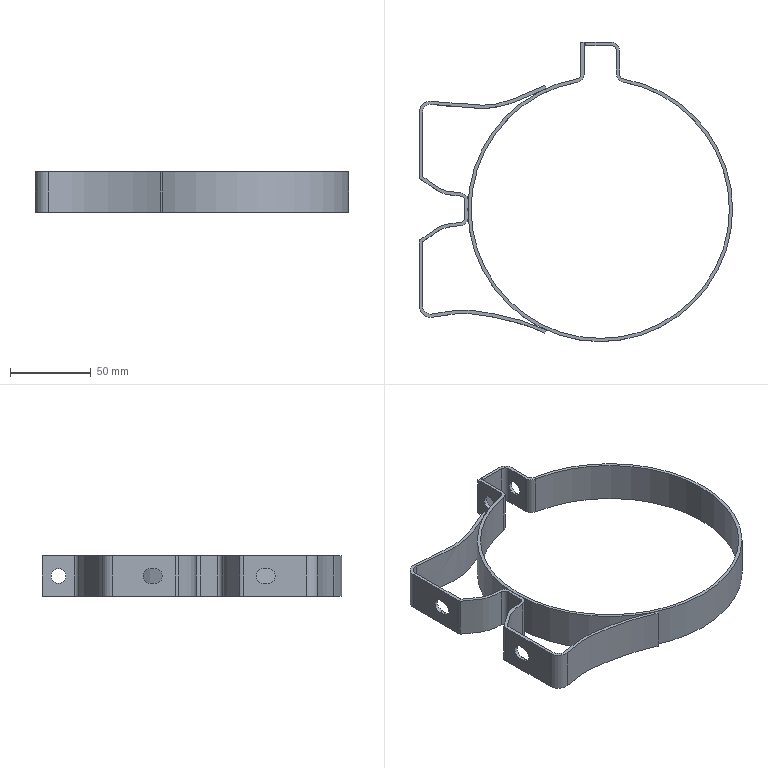Part | SolidWorks | features BaseBody 2 | 2 solids | 64 faces | box 194 x 185.373 x 25 mm | volume 43057 mm3 | cylinder 32 | plane 24 | spline 8 | commonest cylinder face diameters 10 x9 9 x8 6 x5 14 x4 160 x3 164 x3